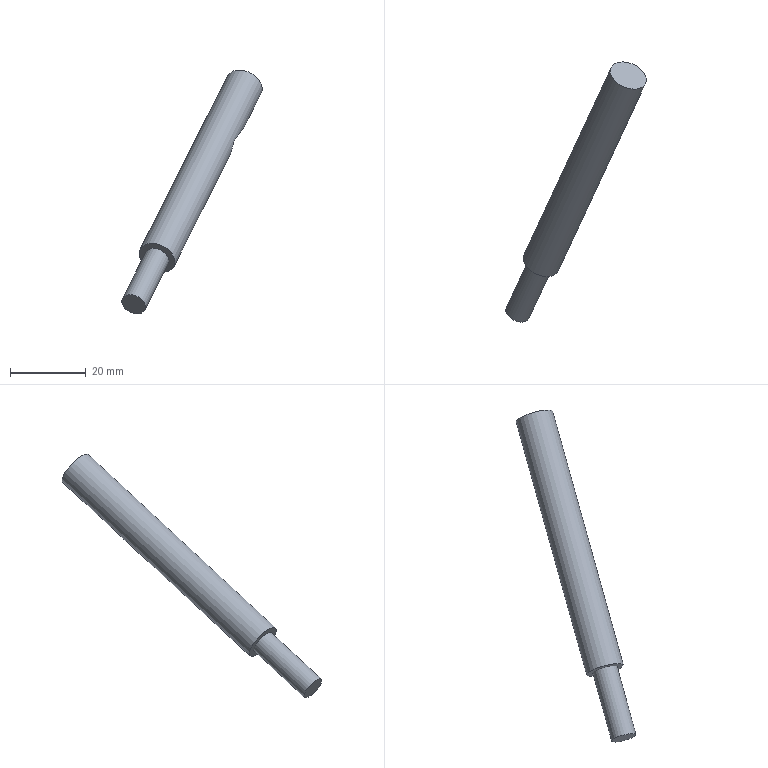Part | NX | features solid 2 | 1 solid | 8 faces | box 36.99 x 68.458 x 64.209 mm | volume 5979 mm3 | plane 3 | cylinder 2 | sphere 2 | cone 1 | commonest cylinder face diameters 6.6 x1 10 x1
STEP:
#1=CARTESIAN_POINT('',(449.302,396.458,-47.58));
#2=VERTEX_POINT('',#1);
#3=CARTESIAN_POINT('',(452.493,406.396,-42.419));
#4=VERTEX_POINT('',#3);
#5=CARTESIAN_POINT('',(449.302,396.458,-47.58));
#6=CARTESIAN_POINT('',(450.659,399.737,-45.99));
#7=CARTESIAN_POINT('',(451.691,403.084,-44.29));
#8=CARTESIAN_POINT('',(452.493,406.396,-42.419));
#9=B_SPLINE_CURVE_WITH_KNOTS('',3,(#5,#6,#7,#8),.UNSPECIFIED.,.F.,.F.,(4,4),(0.000000208,0.01165),.UNSPECIFIED.);
#10=EDGE_CURVE('',#2,#4,#9,.T.);
#11=ORIENTED_EDGE('',*,*,#10,.T.);
#12=CARTESIAN_POINT('',(450.627,408.285,-43.52));
#13=VERTEX_POINT('',#12);
#14=CARTESIAN_POINT('',(452.493,406.396,-42.419));
#15=CARTESIAN_POINT('',(452.63,406.964,-42.099));
#16=CARTESIAN_POINT('',(452.338,408.564,-42.185));
#17=CARTESIAN_POINT('',(450.974,408.641,-43.076));
#18=CARTESIAN_POINT('',(450.627,408.285,-43.52));
#19=B_SPLINE_CURVE_WITH_KNOTS('',3,(#14,#15,#16,#17,#18),.UNSPECIFIED.,.F.,.F.,(4,1,4),(0.000000204,0.001971,0.003941),.UNSPECIFIED.);
#20=EDGE_CURVE('',#4,#13,#19,.T.);
#21=ORIENTED_EDGE('',*,*,#20,.T.);
#22=CARTESIAN_POINT('',(444.211,401.613,-50.584));
#23=VERTEX_POINT('',#22);
#24=CARTESIAN_POINT('',(450.627,408.285,-43.52));
#25=CARTESIAN_POINT('',(448.604,406.208,-46.112));
#26=CARTESIAN_POINT('',(446.433,404.019,-48.483));
#27=CARTESIAN_POINT('',(444.211,401.613,-50.584));
#28=B_SPLINE_CURVE_WITH_KNOTS('',3,(#24,#25,#26,#27),.UNSPECIFIED.,.F.,.F.,(4,4),(0.000000207,0.01167),.UNSPECIFIED.);
#29=EDGE_CURVE('',#13,#23,#28,.T.);
#30=ORIENTED_EDGE('',*,*,#29,.T.);
#31=CARTESIAN_POINT('',(444.211,401.613,-50.584));
#32=CARTESIAN_POINT('',(443.812,401.182,-50.961));
#33=CARTESIAN_POINT('',(443.322,400.201,-51.863));
#34=CARTESIAN_POINT('',(443.643,398.711,-53.365));
#35=CARTESIAN_POINT('',(444.79,397.187,-54.328));
#36=CARTESIAN_POINT('',(446.287,395.627,-54.171));
#37=CARTESIAN_POINT('',(447.474,394.467,-52.754));
#38=CARTESIAN_POINT('',(448.119,394.179,-50.724));
#39=CARTESIAN_POINT('',(448.59,394.858,-48.76));
#40=CARTESIAN_POINT('',(449.058,395.868,-47.865));
#41=CARTESIAN_POINT('',(449.302,396.458,-47.58));
#42=B_SPLINE_CURVE_WITH_KNOTS('',3,(#31,#32,#33,#34,#35,#36,#37,#38,#39,#40,#41),.UNSPECIFIED.,.F.,.F.,(4,1,1,1,1,1,1,1,4),(0.000000205,0.002065,0.00413,0.006195,0.00826,0.01033,0.01239,0.01446,0.01652),.UNSPECIFIED.);
#43=EDGE_CURVE('',#23,#2,#42,.T.);
#44=ORIENTED_EDGE('',*,*,#43,.T.);
#45=EDGE_LOOP('',(#11,#21,#30,#44));
#46=FACE_BOUND('',#45,.T.);
#47=CARTESIAN_POINT('',(454.625,409.333,-31.691));
#48=VERTEX_POINT('',#47);
#49=CARTESIAN_POINT('',(451.379,412.619,-33.606));
#50=DIRECTION('',(0.3237,0.6943,0.6428));
#51=DIRECTION('',(0.6491,-0.6573,0.383));
#52=AXIS2_PLACEMENT_3D('',#49,#50,#51);
#53=CIRCLE('',#52,5.);
#54=EDGE_CURVE('',#48,#48,#53,.T.);
#55=ORIENTED_EDGE('',*,*,#54,.F.);
#56=EDGE_LOOP('',(#55));
#57=FACE_BOUND('',#56,.T.);
#58=CARTESIAN_POINT('',(431.639,360.039,-77.329));
#59=VERTEX_POINT('',#58);
#60=CARTESIAN_POINT('',(428.393,363.326,-79.244));
#61=DIRECTION('',(0.3237,0.6943,0.6428));
#62=DIRECTION('',(0.6491,-0.6573,0.383));
#63=AXIS2_PLACEMENT_3D('',#60,#61,#62);
#64=CIRCLE('',#63,5.);
#65=EDGE_CURVE('',#59,#59,#64,.T.);
#66=ORIENTED_EDGE('',*,*,#65,.T.);
#67=EDGE_LOOP('',(#66));
#68=FACE_BOUND('',#67,.T.);
#69=CARTESIAN_POINT('',(451.379,412.619,-33.606));
#70=DIRECTION('',(-0.3237,-0.6943,-0.6428));
#71=DIRECTION('',(-0.6491,0.6573,-0.383));
#72=AXIS2_PLACEMENT_3D('',#69,#70,#71);
#73=CYLINDRICAL_SURFACE('',#72,5.);
#74=ADVANCED_FACE('',(#46,#57,#68),#73,.T.);
#75=ORIENTED_EDGE('',*,*,#54,.T.);
#76=EDGE_LOOP('',(#75));
#77=FACE_BOUND('',#76,.T.);
#78=CARTESIAN_POINT('',(451.379,412.619,-33.606));
#79=DIRECTION('',(0.3237,0.6943,0.6428));
#80=DIRECTION('',(0.6491,-0.6573,0.383));
#81=AXIS2_PLACEMENT_3D('',#78,#79,#80);
#82=PLANE('',#81);
#83=ADVANCED_FACE('',(#77),#82,.T.);
#84=CARTESIAN_POINT('',(430.535,361.157,-77.98));
#85=VERTEX_POINT('',#84);
#86=CARTESIAN_POINT('',(428.393,363.326,-79.244));
#87=DIRECTION('',(0.3237,0.6943,0.6428));
#88=DIRECTION('',(0.6491,-0.6573,0.383));
#89=AXIS2_PLACEMENT_3D('',#86,#87,#88);
#90=CIRCLE('',#89,3.3);
#91=EDGE_CURVE('',#85,#85,#90,.T.);
#92=ORIENTED_EDGE('',*,*,#91,.T.);
#93=EDGE_LOOP('',(#92));
#94=FACE_BOUND('',#93,.T.);
#95=ORIENTED_EDGE('',*,*,#65,.F.);
#96=EDGE_LOOP('',(#95));
#97=FACE_BOUND('',#96,.T.);
#98=CARTESIAN_POINT('',(428.393,363.326,-79.244));
#99=DIRECTION('',(0.3237,0.6943,0.6428));
#100=DIRECTION('',(0.6491,-0.6573,0.383));
#101=AXIS2_PLACEMENT_3D('',#98,#99,#100);
#102=PLANE('',#101);
#103=ADVANCED_FACE('',(#94,#97),#102,.F.);
#104=CARTESIAN_POINT('',(424.384,347.966,-90.193));
#105=VERTEX_POINT('',#104);
#106=CARTESIAN_POINT('',(422.242,350.135,-91.457));
#107=DIRECTION('',(0.3237,0.6943,0.6428));
#108=DIRECTION('',(0.6491,-0.6573,0.383));
#109=AXIS2_PLACEMENT_3D('',#106,#107,#108);
#110=CIRCLE('',#109,3.3);
#111=EDGE_CURVE('',#105,#105,#110,.T.);
#112=ORIENTED_EDGE('',*,*,#111,.T.);
#113=EDGE_LOOP('',(#112));
#114=FACE_BOUND('',#113,.T.);
#115=ORIENTED_EDGE('',*,*,#91,.F.);
#116=EDGE_LOOP('',(#115));
#117=FACE_BOUND('',#116,.T.);
#118=CARTESIAN_POINT('',(422.242,350.135,-91.457));
#119=DIRECTION('',(0.3237,0.6943,0.6428));
#120=DIRECTION('',(0.6491,-0.6573,0.383));
#121=AXIS2_PLACEMENT_3D('',#118,#119,#120);
#122=CYLINDRICAL_SURFACE('',#121,3.3);
#123=ADVANCED_FACE('',(#114,#117),#122,.T.);
#124=ORIENTED_EDGE('',*,*,#111,.F.);
#125=EDGE_LOOP('',(#124));
#126=FACE_BOUND('',#125,.T.);
#127=CARTESIAN_POINT('',(422.242,350.135,-91.457));
#128=DIRECTION('',(0.3237,0.6943,0.6428));
#129=DIRECTION('',(0.6491,-0.6573,0.383));
#130=AXIS2_PLACEMENT_3D('',#127,#128,#129);
#131=PLANE('',#130);
#132=ADVANCED_FACE('',(#126),#131,.F.);
#133=CARTESIAN_POINT('',(448.063,399.592,-50.341));
#134=DIRECTION('',(-0.3237,-0.6943,-0.6428));
#135=DIRECTION('',(-0.6491,0.6573,-0.383));
#136=AXIS2_PLACEMENT_3D('',#133,#134,#135);
#137=CIRCLE('',#136,4.357);
#138=EDGE_CURVE('',#2,#23,#137,.T.);
#139=ORIENTED_EDGE('',*,*,#138,.F.);
#140=ORIENTED_EDGE('',*,*,#43,.F.);
#141=EDGE_LOOP('',(#139,#140));
#142=FACE_BOUND('',#141,.T.);
#143=CARTESIAN_POINT('',(447.699,398.811,-51.064));
#144=DIRECTION('',(-0.3237,-0.6943,-0.6428));
#145=DIRECTION('',(-0.6491,0.6573,-0.383));
#146=AXIS2_PLACEMENT_3D('',#143,#144,#145);
#147=SPHERICAL_SURFACE('',#146,4.5);
#148=ADVANCED_FACE('',(#142),#147,.F.);
#149=CARTESIAN_POINT('',(451.705,407.403,-43.11));
#150=DIRECTION('',(-0.3237,-0.6943,-0.6428));
#151=DIRECTION('',(-0.6491,0.6573,-0.383));
#152=AXIS2_PLACEMENT_3D('',#149,#150,#151);
#153=CIRCLE('',#152,1.452);
#154=EDGE_CURVE('',#4,#13,#153,.T.);
#155=ORIENTED_EDGE('',*,*,#154,.F.);
#156=ORIENTED_EDGE('',*,*,#10,.F.);
#157=ORIENTED_EDGE('',*,*,#138,.T.);
#158=ORIENTED_EDGE('',*,*,#29,.F.);
#159=EDGE_LOOP('',(#155,#156,#157,#158));
#160=FACE_BOUND('',#159,.T.);
#161=CARTESIAN_POINT('',(448.063,399.592,-50.341));
#162=DIRECTION('',(-0.3237,-0.6943,-0.6428));
#163=DIRECTION('',(-0.6491,0.6573,-0.383));
#164=AXIS2_PLACEMENT_3D('',#161,#162,#163);
#165=CONICAL_SURFACE('',#164,4.357,0.2527);
#166=ADVANCED_FACE('',(#160),#165,.F.);
#167=ORIENTED_EDGE('',*,*,#154,.T.);
#168=ORIENTED_EDGE('',*,*,#20,.F.);
#169=EDGE_LOOP('',(#167,#168));
#170=FACE_BOUND('',#169,.T.);
#171=CARTESIAN_POINT('',(451.584,407.142,-43.351));
#172=DIRECTION('',(-0.3237,-0.6943,-0.6428));
#173=DIRECTION('',(0.6491,-0.6573,0.383));
#174=AXIS2_PLACEMENT_3D('',#171,#172,#173);
#175=SPHERICAL_SURFACE('',#174,1.5);
#176=ADVANCED_FACE('',(#170),#175,.F.);
#177=CLOSED_SHELL('',(#74,#83,#103,#123,#132,#148,#166,#176));
#178=MANIFOLD_SOLID_BREP('',#177);
#179=(LENGTH_UNIT()NAMED_UNIT(*)SI_UNIT(.MILLI.,.METRE.));
#180=UNCERTAINTY_MEASURE_WITH_UNIT(LENGTH_MEASURE(0.0508),#179,'','');
#181=(NAMED_UNIT(*)PLANE_ANGLE_UNIT()SI_UNIT($,.RADIAN.));
#182=(NAMED_UNIT(*)SI_UNIT($,.STERADIAN.)SOLID_ANGLE_UNIT());
#183=(GEOMETRIC_REPRESENTATION_CONTEXT(3)GLOBAL_UNCERTAINTY_ASSIGNED_CONTEXT((#180))GLOBAL_UNIT_ASSIGNED_CONTEXT((#179,#181,#182))REPRESENTATION_CONTEXT('',''));
#184=ADVANCED_BREP_SHAPE_REPRESENTATION('',(#178),#183);